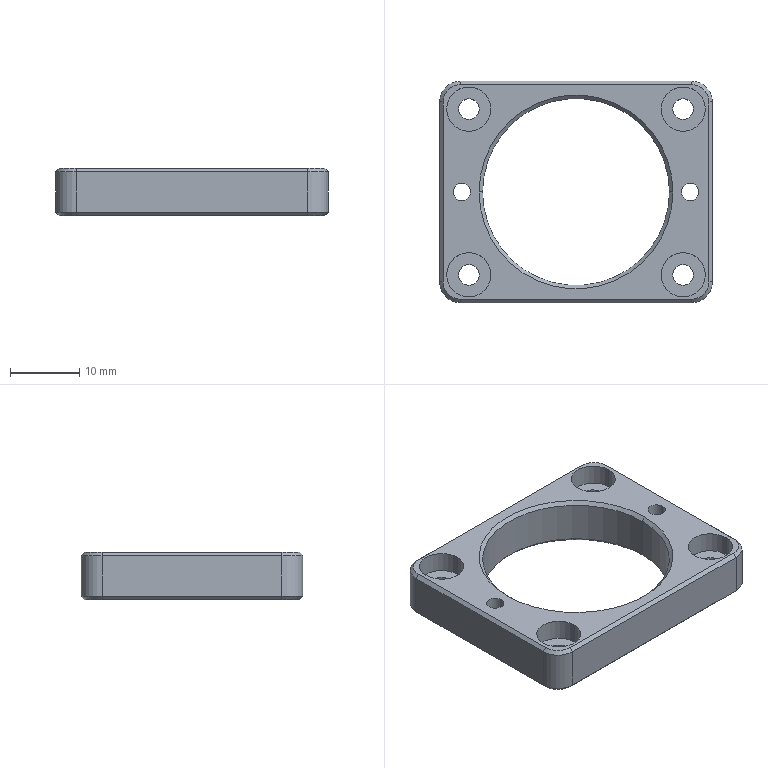Part | NX | features BREP 1 | 1 solid | 56 faces | box 39.409 x 32 x 6.9 mm | volume 4078 mm3 | cylinder 26 | plane 18 | cone 12 | commonest cylinder face diameters 3 x8 6.4 x8 2.5 x4 6 x4 27 x2